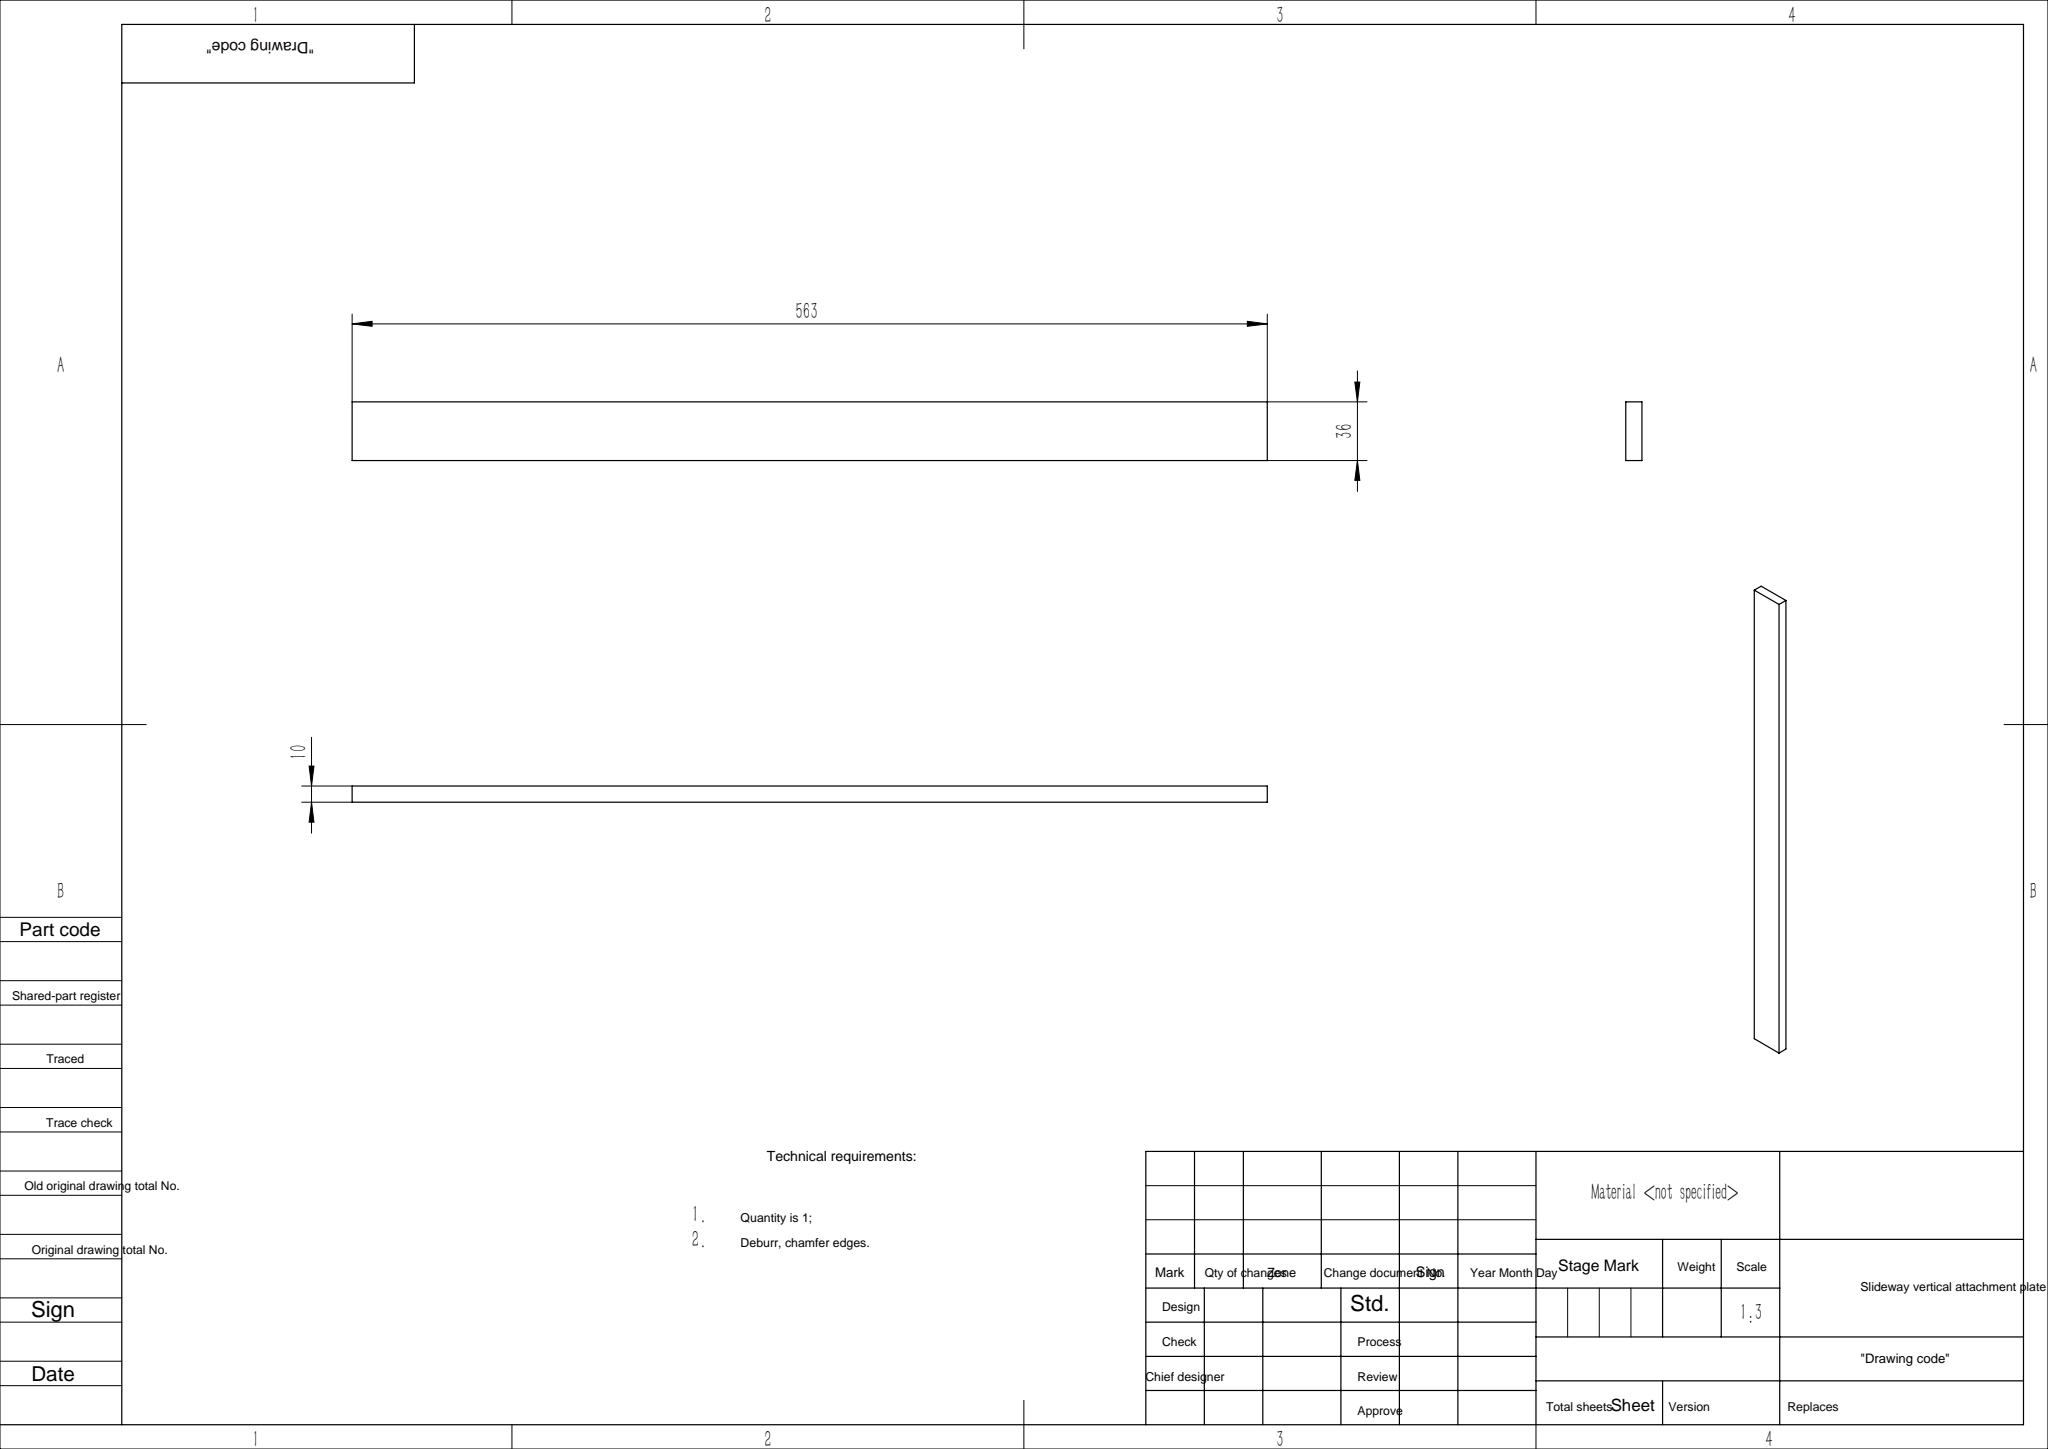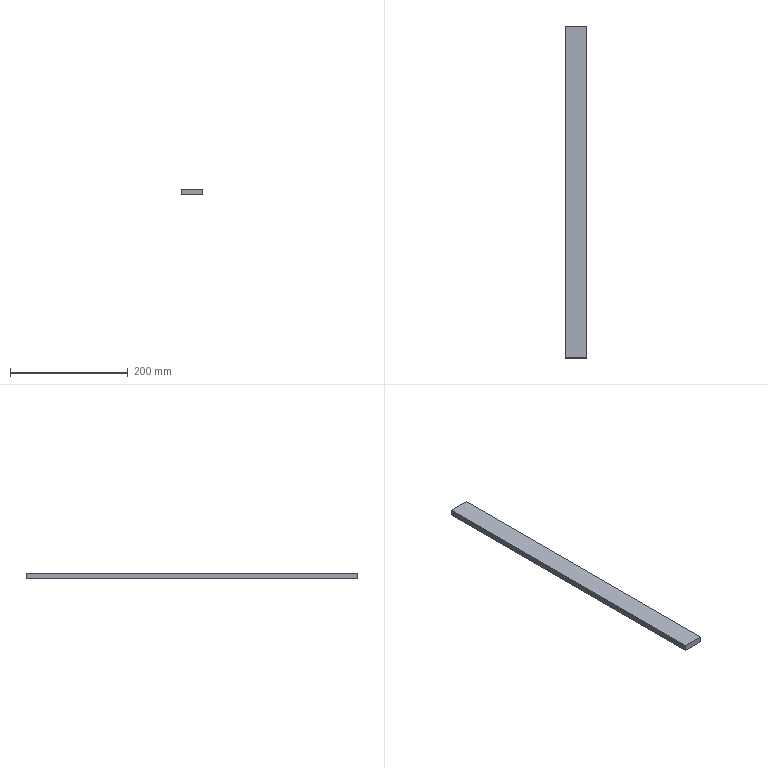Part | SolidWorks | features Extrusion 1 | 1 solid | 6 faces | box 36 x 563 x 10 mm | volume 202680 mm3 | plane 6
STEP:
#1=CARTESIAN_POINT('',(-18.,30.,-20.));
#2=VERTEX_POINT('',#1);
#3=CARTESIAN_POINT('',(-18.,30.,-10.));
#4=VERTEX_POINT('',#3);
#5=CARTESIAN_POINT('',(-18.,30.,-10.));
#6=DIRECTION('',(0.,0.,1.));
#7=VECTOR('',#6,1000.);
#8=LINE('',#5,#7);
#9=EDGE_CURVE('',#2,#4,#8,.T.);
#10=ORIENTED_EDGE('',*,*,#9,.T.);
#11=CARTESIAN_POINT('',(-18.,593.,-10.));
#12=VERTEX_POINT('',#11);
#13=CARTESIAN_POINT('',(-18.,593.,-10.));
#14=DIRECTION('',(0.,-1.,0.));
#15=VECTOR('',#14,1000.);
#16=LINE('',#13,#15);
#17=EDGE_CURVE('',#12,#4,#16,.T.);
#18=ORIENTED_EDGE('',*,*,#17,.F.);
#19=CARTESIAN_POINT('',(-18.,593.,-20.));
#20=VERTEX_POINT('',#19);
#21=CARTESIAN_POINT('',(-18.,593.,-10.));
#22=DIRECTION('',(0.,0.,1.));
#23=VECTOR('',#22,1000.);
#24=LINE('',#21,#23);
#25=EDGE_CURVE('',#20,#12,#24,.T.);
#26=ORIENTED_EDGE('',*,*,#25,.F.);
#27=CARTESIAN_POINT('',(-18.,593.,-20.));
#28=DIRECTION('',(0.,-1.,0.));
#29=VECTOR('',#28,1000.);
#30=LINE('',#27,#29);
#31=EDGE_CURVE('',#20,#2,#30,.T.);
#32=ORIENTED_EDGE('',*,*,#31,.T.);
#33=EDGE_LOOP('',(#10,#18,#26,#32));
#34=FACE_OUTER_BOUND('',#33,.T.);
#35=CARTESIAN_POINT('',(-18.,593.,-10.));
#36=DIRECTION('',(1.,0.,0.));
#37=DIRECTION('',(0.,0.,-1.));
#38=AXIS2_PLACEMENT_3D('',#35,#36,#37);
#39=PLANE('',#38);
#40=ADVANCED_FACE('',(#34),#39,.F.);
#41=CARTESIAN_POINT('',(18.,30.,-10.));
#42=VERTEX_POINT('',#41);
#43=CARTESIAN_POINT('',(-18.,30.,-10.));
#44=DIRECTION('',(1.,0.,0.));
#45=VECTOR('',#44,1000.);
#46=LINE('',#43,#45);
#47=EDGE_CURVE('',#4,#42,#46,.T.);
#48=ORIENTED_EDGE('',*,*,#47,.T.);
#49=CARTESIAN_POINT('',(18.,593.,-10.));
#50=VERTEX_POINT('',#49);
#51=CARTESIAN_POINT('',(18.,593.,-10.));
#52=DIRECTION('',(0.,-1.,0.));
#53=VECTOR('',#52,1000.);
#54=LINE('',#51,#53);
#55=EDGE_CURVE('',#50,#42,#54,.T.);
#56=ORIENTED_EDGE('',*,*,#55,.F.);
#57=CARTESIAN_POINT('',(-18.,593.,-10.));
#58=DIRECTION('',(1.,0.,0.));
#59=VECTOR('',#58,1000.);
#60=LINE('',#57,#59);
#61=EDGE_CURVE('',#12,#50,#60,.T.);
#62=ORIENTED_EDGE('',*,*,#61,.F.);
#63=ORIENTED_EDGE('',*,*,#17,.T.);
#64=EDGE_LOOP('',(#48,#56,#62,#63));
#65=FACE_OUTER_BOUND('',#64,.T.);
#66=CARTESIAN_POINT('',(-18.,593.,-10.));
#67=DIRECTION('',(0.,0.,-1.));
#68=DIRECTION('',(-1.,0.,0.));
#69=AXIS2_PLACEMENT_3D('',#66,#67,#68);
#70=PLANE('',#69);
#71=ADVANCED_FACE('',(#65),#70,.F.);
#72=CARTESIAN_POINT('',(18.,30.,-20.));
#73=VERTEX_POINT('',#72);
#74=CARTESIAN_POINT('',(18.,30.,-10.));
#75=DIRECTION('',(0.,0.,-1.));
#76=VECTOR('',#75,1000.);
#77=LINE('',#74,#76);
#78=EDGE_CURVE('',#42,#73,#77,.T.);
#79=ORIENTED_EDGE('',*,*,#78,.T.);
#80=CARTESIAN_POINT('',(18.,593.,-20.));
#81=VERTEX_POINT('',#80);
#82=CARTESIAN_POINT('',(18.,593.,-20.));
#83=DIRECTION('',(0.,-1.,0.));
#84=VECTOR('',#83,1000.);
#85=LINE('',#82,#84);
#86=EDGE_CURVE('',#81,#73,#85,.T.);
#87=ORIENTED_EDGE('',*,*,#86,.F.);
#88=CARTESIAN_POINT('',(18.,593.,-10.));
#89=DIRECTION('',(0.,0.,-1.));
#90=VECTOR('',#89,1000.);
#91=LINE('',#88,#90);
#92=EDGE_CURVE('',#50,#81,#91,.T.);
#93=ORIENTED_EDGE('',*,*,#92,.F.);
#94=ORIENTED_EDGE('',*,*,#55,.T.);
#95=EDGE_LOOP('',(#79,#87,#93,#94));
#96=FACE_OUTER_BOUND('',#95,.T.);
#97=CARTESIAN_POINT('',(18.,593.,-10.));
#98=DIRECTION('',(-1.,0.,0.));
#99=DIRECTION('',(0.,0.,1.));
#100=AXIS2_PLACEMENT_3D('',#97,#98,#99);
#101=PLANE('',#100);
#102=ADVANCED_FACE('',(#96),#101,.F.);
#103=CARTESIAN_POINT('',(-18.,30.,-20.));
#104=DIRECTION('',(-1.,0.,0.));
#105=VECTOR('',#104,1000.);
#106=LINE('',#103,#105);
#107=EDGE_CURVE('',#73,#2,#106,.T.);
#108=ORIENTED_EDGE('',*,*,#107,.T.);
#109=ORIENTED_EDGE('',*,*,#31,.F.);
#110=CARTESIAN_POINT('',(-18.,593.,-20.));
#111=DIRECTION('',(-1.,0.,0.));
#112=VECTOR('',#111,1000.);
#113=LINE('',#110,#112);
#114=EDGE_CURVE('',#81,#20,#113,.T.);
#115=ORIENTED_EDGE('',*,*,#114,.F.);
#116=ORIENTED_EDGE('',*,*,#86,.T.);
#117=EDGE_LOOP('',(#108,#109,#115,#116));
#118=FACE_OUTER_BOUND('',#117,.T.);
#119=CARTESIAN_POINT('',(-18.,593.,-20.));
#120=DIRECTION('',(0.,0.,1.));
#121=DIRECTION('',(1.,0.,0.));
#122=AXIS2_PLACEMENT_3D('',#119,#120,#121);
#123=PLANE('',#122);
#124=ADVANCED_FACE('',(#118),#123,.F.);
#125=ORIENTED_EDGE('',*,*,#25,.T.);
#126=ORIENTED_EDGE('',*,*,#61,.T.);
#127=ORIENTED_EDGE('',*,*,#92,.T.);
#128=ORIENTED_EDGE('',*,*,#114,.T.);
#129=EDGE_LOOP('',(#125,#126,#127,#128));
#130=FACE_OUTER_BOUND('',#129,.T.);
#131=CARTESIAN_POINT('',(0.,593.,0.));
#132=DIRECTION('',(0.,-1.,0.));
#133=DIRECTION('',(0.,0.,-1.));
#134=AXIS2_PLACEMENT_3D('',#131,#132,#133);
#135=PLANE('',#134);
#136=ADVANCED_FACE('',(#130),#135,.F.);
#137=ORIENTED_EDGE('',*,*,#9,.F.);
#138=ORIENTED_EDGE('',*,*,#107,.F.);
#139=ORIENTED_EDGE('',*,*,#78,.F.);
#140=ORIENTED_EDGE('',*,*,#47,.F.);
#141=EDGE_LOOP('',(#137,#138,#139,#140));
#142=FACE_OUTER_BOUND('',#141,.T.);
#143=CARTESIAN_POINT('',(0.,30.,0.));
#144=DIRECTION('',(0.,-1.,0.));
#145=DIRECTION('',(0.,0.,-1.));
#146=AXIS2_PLACEMENT_3D('',#143,#144,#145);
#147=PLANE('',#146);
#148=ADVANCED_FACE('',(#142),#147,.T.);
#149=CLOSED_SHELL('',(#40,#71,#102,#124,#136,#148));
#150=MANIFOLD_SOLID_BREP('',#149);
#151=CARTESIAN_POINT('',(0.,0.,0.));
#152=DIRECTION('',(0.,0.,1.));
#153=DIRECTION('',(1.,0.,0.));
#154=AXIS2_PLACEMENT_3D('',#151,#152,#153);
#155=(LENGTH_UNIT()NAMED_UNIT(*)SI_UNIT(.MILLI.,.METRE.));
#156=UNCERTAINTY_MEASURE_WITH_UNIT(LENGTH_MEASURE(0.00001),#155,'','');
#157=(NAMED_UNIT(*)PLANE_ANGLE_UNIT()SI_UNIT($,.RADIAN.));
#158=(NAMED_UNIT(*)SI_UNIT($,.STERADIAN.)SOLID_ANGLE_UNIT());
#159=(GEOMETRIC_REPRESENTATION_CONTEXT(3)GLOBAL_UNCERTAINTY_ASSIGNED_CONTEXT((#156))GLOBAL_UNIT_ASSIGNED_CONTEXT((#155,#157,#158))REPRESENTATION_CONTEXT('',''));
#160=ADVANCED_BREP_SHAPE_REPRESENTATION('',(#150,#154),#159);